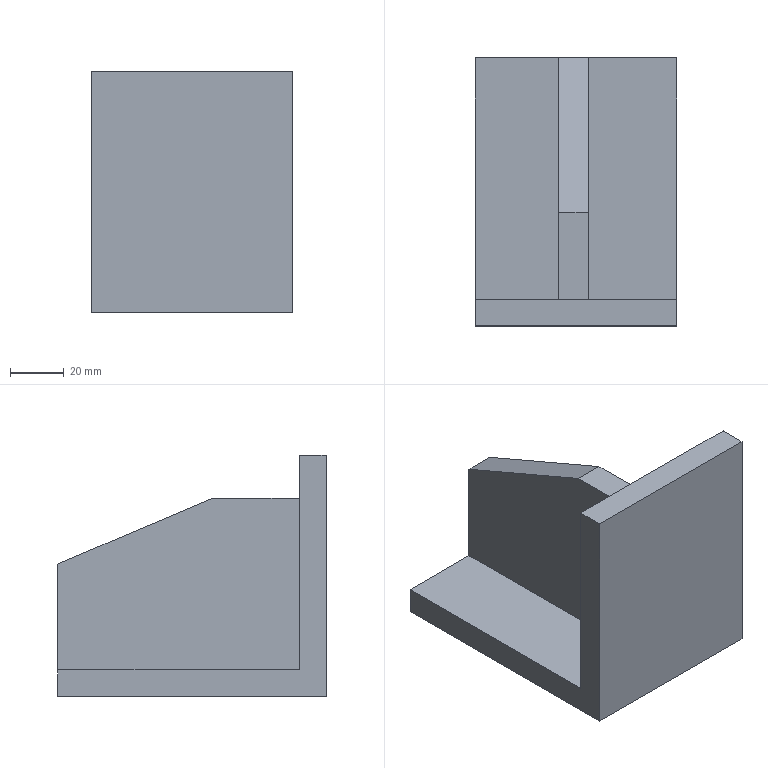Part | STEP file | MYT-A01-P39 | 1 solid | 13 faces | box 75 x 100 x 90 mm | volume 190302 mm3 | plane 13
STEP:
#1=CARTESIAN_POINT('',(-6.413,-40.,10.));
#2=VERTEX_POINT('',#1);
#3=CARTESIAN_POINT('',(-37.5,-40.,10.));
#4=VERTEX_POINT('',#3);
#5=CARTESIAN_POINT('',(-37.5,-40.,10.));
#6=DIRECTION('',(-1.,0.,0.));
#7=VECTOR('',#6,1000.);
#8=LINE('',#5,#7);
#9=EDGE_CURVE('',#2,#4,#8,.T.);
#10=ORIENTED_EDGE('',*,*,#9,.F.);
#11=CARTESIAN_POINT('',(-6.413,50.,10.));
#12=VERTEX_POINT('',#11);
#13=CARTESIAN_POINT('',(-6.413,50.,10.));
#14=DIRECTION('',(0.,-1.,0.));
#15=VECTOR('',#14,1000.);
#16=LINE('',#13,#15);
#17=EDGE_CURVE('',#12,#2,#16,.T.);
#18=ORIENTED_EDGE('',*,*,#17,.F.);
#19=CARTESIAN_POINT('',(-37.5,50.,10.));
#20=VERTEX_POINT('',#19);
#21=CARTESIAN_POINT('',(-37.5,50.,10.));
#22=DIRECTION('',(-1.,0.,0.));
#23=VECTOR('',#22,1000.);
#24=LINE('',#21,#23);
#25=EDGE_CURVE('',#12,#20,#24,.T.);
#26=ORIENTED_EDGE('',*,*,#25,.T.);
#27=CARTESIAN_POINT('',(-37.5,50.,10.));
#28=DIRECTION('',(0.,-1.,0.));
#29=VECTOR('',#28,1000.);
#30=LINE('',#27,#29);
#31=EDGE_CURVE('',#20,#4,#30,.T.);
#32=ORIENTED_EDGE('',*,*,#31,.T.);
#33=EDGE_LOOP('',(#10,#18,#26,#32));
#34=FACE_OUTER_BOUND('',#33,.T.);
#35=CARTESIAN_POINT('',(0.,0.,10.));
#36=DIRECTION('',(0.,0.,1.));
#37=DIRECTION('',(1.,0.,0.));
#38=AXIS2_PLACEMENT_3D('',#35,#36,#37);
#39=PLANE('',#38);
#40=ADVANCED_FACE('',(#34),#39,.T.);
#41=CARTESIAN_POINT('',(37.5,50.,10.));
#42=VERTEX_POINT('',#41);
#43=CARTESIAN_POINT('',(4.531,50.,10.));
#44=VERTEX_POINT('',#43);
#45=CARTESIAN_POINT('',(-37.5,50.,10.));
#46=DIRECTION('',(-1.,0.,0.));
#47=VECTOR('',#46,1000.);
#48=LINE('',#45,#47);
#49=EDGE_CURVE('',#42,#44,#48,.T.);
#50=ORIENTED_EDGE('',*,*,#49,.T.);
#51=CARTESIAN_POINT('',(4.531,-40.,10.));
#52=VERTEX_POINT('',#51);
#53=CARTESIAN_POINT('',(4.531,50.,10.));
#54=DIRECTION('',(0.,1.,0.));
#55=VECTOR('',#54,1000.);
#56=LINE('',#53,#55);
#57=EDGE_CURVE('',#52,#44,#56,.T.);
#58=ORIENTED_EDGE('',*,*,#57,.F.);
#59=CARTESIAN_POINT('',(37.5,-40.,10.));
#60=VERTEX_POINT('',#59);
#61=CARTESIAN_POINT('',(-37.5,-40.,10.));
#62=DIRECTION('',(-1.,0.,0.));
#63=VECTOR('',#62,1000.);
#64=LINE('',#61,#63);
#65=EDGE_CURVE('',#60,#52,#64,.T.);
#66=ORIENTED_EDGE('',*,*,#65,.F.);
#67=CARTESIAN_POINT('',(37.5,50.,10.));
#68=DIRECTION('',(0.,1.,0.));
#69=VECTOR('',#68,1000.);
#70=LINE('',#67,#69);
#71=EDGE_CURVE('',#60,#42,#70,.T.);
#72=ORIENTED_EDGE('',*,*,#71,.T.);
#73=EDGE_LOOP('',(#50,#58,#66,#72));
#74=FACE_OUTER_BOUND('',#73,.T.);
#75=CARTESIAN_POINT('',(0.,0.,10.));
#76=DIRECTION('',(0.,0.,1.));
#77=DIRECTION('',(1.,0.,0.));
#78=AXIS2_PLACEMENT_3D('',#75,#76,#77);
#79=PLANE('',#78);
#80=ADVANCED_FACE('',(#74),#79,.T.);
#81=CARTESIAN_POINT('',(-6.413,-40.,74.));
#82=VERTEX_POINT('',#81);
#83=CARTESIAN_POINT('',(-6.413,-40.,74.));
#84=DIRECTION('',(0.,0.,-1.));
#85=VECTOR('',#84,1000.);
#86=LINE('',#83,#85);
#87=EDGE_CURVE('',#82,#2,#86,.T.);
#88=ORIENTED_EDGE('',*,*,#87,.T.);
#89=ORIENTED_EDGE('',*,*,#9,.T.);
#90=CARTESIAN_POINT('',(-37.5,-40.,90.));
#91=VERTEX_POINT('',#90);
#92=CARTESIAN_POINT('',(-37.5,-40.,90.));
#93=DIRECTION('',(0.,0.,-1.));
#94=VECTOR('',#93,1000.);
#95=LINE('',#92,#94);
#96=EDGE_CURVE('',#91,#4,#95,.T.);
#97=ORIENTED_EDGE('',*,*,#96,.F.);
#98=CARTESIAN_POINT('',(37.5,-40.,90.));
#99=VERTEX_POINT('',#98);
#100=CARTESIAN_POINT('',(-37.5,-40.,90.));
#101=DIRECTION('',(-1.,0.,0.));
#102=VECTOR('',#101,1000.);
#103=LINE('',#100,#102);
#104=EDGE_CURVE('',#99,#91,#103,.T.);
#105=ORIENTED_EDGE('',*,*,#104,.F.);
#106=CARTESIAN_POINT('',(37.5,-40.,90.));
#107=DIRECTION('',(0.,0.,-1.));
#108=VECTOR('',#107,1000.);
#109=LINE('',#106,#108);
#110=EDGE_CURVE('',#99,#60,#109,.T.);
#111=ORIENTED_EDGE('',*,*,#110,.T.);
#112=ORIENTED_EDGE('',*,*,#65,.T.);
#113=CARTESIAN_POINT('',(4.531,-40.,74.));
#114=VERTEX_POINT('',#113);
#115=CARTESIAN_POINT('',(4.531,-40.,74.));
#116=DIRECTION('',(0.,0.,-1.));
#117=VECTOR('',#116,1000.);
#118=LINE('',#115,#117);
#119=EDGE_CURVE('',#114,#52,#118,.T.);
#120=ORIENTED_EDGE('',*,*,#119,.F.);
#121=CARTESIAN_POINT('',(-6.413,-40.,74.));
#122=DIRECTION('',(1.,0.,0.));
#123=VECTOR('',#122,1000.);
#124=LINE('',#121,#123);
#125=EDGE_CURVE('',#82,#114,#124,.T.);
#126=ORIENTED_EDGE('',*,*,#125,.F.);
#127=EDGE_LOOP('',(#88,#89,#97,#105,#111,#112,#120,#126));
#128=FACE_OUTER_BOUND('',#127,.T.);
#129=CARTESIAN_POINT('',(-37.5,-40.,90.));
#130=DIRECTION('',(0.,-1.,0.));
#131=DIRECTION('',(0.,0.,-1.));
#132=AXIS2_PLACEMENT_3D('',#129,#130,#131);
#133=PLANE('',#132);
#134=ADVANCED_FACE('',(#128),#133,.F.);
#135=CARTESIAN_POINT('',(37.5,-50.,0.));
#136=VERTEX_POINT('',#135);
#137=CARTESIAN_POINT('',(37.5,50.,0.));
#138=VERTEX_POINT('',#137);
#139=CARTESIAN_POINT('',(37.5,50.,0.));
#140=DIRECTION('',(0.,1.,0.));
#141=VECTOR('',#140,1000.);
#142=LINE('',#139,#141);
#143=EDGE_CURVE('',#136,#138,#142,.T.);
#144=ORIENTED_EDGE('',*,*,#143,.T.);
#145=CARTESIAN_POINT('',(37.5,50.,10.));
#146=DIRECTION('',(0.,0.,-1.));
#147=VECTOR('',#146,1000.);
#148=LINE('',#145,#147);
#149=EDGE_CURVE('',#42,#138,#148,.T.);
#150=ORIENTED_EDGE('',*,*,#149,.F.);
#151=ORIENTED_EDGE('',*,*,#71,.F.);
#152=ORIENTED_EDGE('',*,*,#110,.F.);
#153=CARTESIAN_POINT('',(37.5,-50.,90.));
#154=VERTEX_POINT('',#153);
#155=CARTESIAN_POINT('',(37.5,-50.,90.));
#156=DIRECTION('',(0.,1.,0.));
#157=VECTOR('',#156,1000.);
#158=LINE('',#155,#157);
#159=EDGE_CURVE('',#154,#99,#158,.T.);
#160=ORIENTED_EDGE('',*,*,#159,.F.);
#161=CARTESIAN_POINT('',(37.5,-50.,10.));
#162=DIRECTION('',(0.,0.,-1.));
#163=VECTOR('',#162,1000.);
#164=LINE('',#161,#163);
#165=EDGE_CURVE('',#154,#136,#164,.T.);
#166=ORIENTED_EDGE('',*,*,#165,.T.);
#167=EDGE_LOOP('',(#144,#150,#151,#152,#160,#166));
#168=FACE_OUTER_BOUND('',#167,.T.);
#169=CARTESIAN_POINT('',(37.5,50.,10.));
#170=DIRECTION('',(-1.,0.,0.));
#171=DIRECTION('',(0.,-1.,0.));
#172=AXIS2_PLACEMENT_3D('',#169,#170,#171);
#173=PLANE('',#172);
#174=ADVANCED_FACE('',(#168),#173,.F.);
#175=CARTESIAN_POINT('',(-6.413,50.,49.448));
#176=VERTEX_POINT('',#175);
#177=CARTESIAN_POINT('',(-6.413,50.,74.));
#178=DIRECTION('',(0.,0.,-1.));
#179=VECTOR('',#178,1000.);
#180=LINE('',#177,#179);
#181=EDGE_CURVE('',#176,#12,#180,.T.);
#182=ORIENTED_EDGE('',*,*,#181,.F.);
#183=CARTESIAN_POINT('',(4.531,50.,49.448));
#184=VERTEX_POINT('',#183);
#185=CARTESIAN_POINT('',(-37.5,50.,49.448));
#186=DIRECTION('',(1.,0.,0.));
#187=VECTOR('',#186,1000.);
#188=LINE('',#185,#187);
#189=EDGE_CURVE('',#176,#184,#188,.T.);
#190=ORIENTED_EDGE('',*,*,#189,.T.);
#191=CARTESIAN_POINT('',(4.531,50.,74.));
#192=DIRECTION('',(0.,0.,-1.));
#193=VECTOR('',#192,1000.);
#194=LINE('',#191,#193);
#195=EDGE_CURVE('',#184,#44,#194,.T.);
#196=ORIENTED_EDGE('',*,*,#195,.T.);
#197=ORIENTED_EDGE('',*,*,#49,.F.);
#198=ORIENTED_EDGE('',*,*,#149,.T.);
#199=CARTESIAN_POINT('',(-37.5,50.,0.));
#200=VERTEX_POINT('',#199);
#201=CARTESIAN_POINT('',(-37.5,50.,0.));
#202=DIRECTION('',(-1.,0.,0.));
#203=VECTOR('',#202,1000.);
#204=LINE('',#201,#203);
#205=EDGE_CURVE('',#138,#200,#204,.T.);
#206=ORIENTED_EDGE('',*,*,#205,.T.);
#207=CARTESIAN_POINT('',(-37.5,50.,10.));
#208=DIRECTION('',(0.,0.,-1.));
#209=VECTOR('',#208,1000.);
#210=LINE('',#207,#209);
#211=EDGE_CURVE('',#20,#200,#210,.T.);
#212=ORIENTED_EDGE('',*,*,#211,.F.);
#213=ORIENTED_EDGE('',*,*,#25,.F.);
#214=EDGE_LOOP('',(#182,#190,#196,#197,#198,#206,#212,#213));
#215=FACE_OUTER_BOUND('',#214,.T.);
#216=CARTESIAN_POINT('',(-37.5,50.,10.));
#217=DIRECTION('',(0.,-1.,0.));
#218=DIRECTION('',(0.,0.,-1.));
#219=AXIS2_PLACEMENT_3D('',#216,#217,#218);
#220=PLANE('',#219);
#221=ADVANCED_FACE('',(#215),#220,.F.);
#222=CARTESIAN_POINT('',(-37.5,-50.,0.));
#223=VERTEX_POINT('',#222);
#224=CARTESIAN_POINT('',(-37.5,50.,0.));
#225=DIRECTION('',(0.,-1.,0.));
#226=VECTOR('',#225,1000.);
#227=LINE('',#224,#226);
#228=EDGE_CURVE('',#200,#223,#227,.T.);
#229=ORIENTED_EDGE('',*,*,#228,.T.);
#230=CARTESIAN_POINT('',(-37.5,-50.,90.));
#231=VERTEX_POINT('',#230);
#232=CARTESIAN_POINT('',(-37.5,-50.,10.));
#233=DIRECTION('',(0.,0.,-1.));
#234=VECTOR('',#233,1000.);
#235=LINE('',#232,#234);
#236=EDGE_CURVE('',#231,#223,#235,.T.);
#237=ORIENTED_EDGE('',*,*,#236,.F.);
#238=CARTESIAN_POINT('',(-37.5,-50.,90.));
#239=DIRECTION('',(0.,-1.,0.));
#240=VECTOR('',#239,1000.);
#241=LINE('',#238,#240);
#242=EDGE_CURVE('',#91,#231,#241,.T.);
#243=ORIENTED_EDGE('',*,*,#242,.F.);
#244=ORIENTED_EDGE('',*,*,#96,.T.);
#245=ORIENTED_EDGE('',*,*,#31,.F.);
#246=ORIENTED_EDGE('',*,*,#211,.T.);
#247=EDGE_LOOP('',(#229,#237,#243,#244,#245,#246));
#248=FACE_OUTER_BOUND('',#247,.T.);
#249=CARTESIAN_POINT('',(-37.5,50.,10.));
#250=DIRECTION('',(1.,0.,0.));
#251=DIRECTION('',(0.,1.,0.));
#252=AXIS2_PLACEMENT_3D('',#249,#250,#251);
#253=PLANE('',#252);
#254=ADVANCED_FACE('',(#248),#253,.F.);
#255=CARTESIAN_POINT('',(-37.5,-50.,0.));
#256=DIRECTION('',(1.,0.,0.));
#257=VECTOR('',#256,1000.);
#258=LINE('',#255,#257);
#259=EDGE_CURVE('',#223,#136,#258,.T.);
#260=ORIENTED_EDGE('',*,*,#259,.T.);
#261=ORIENTED_EDGE('',*,*,#165,.F.);
#262=CARTESIAN_POINT('',(-37.5,-50.,90.));
#263=DIRECTION('',(1.,0.,0.));
#264=VECTOR('',#263,1000.);
#265=LINE('',#262,#264);
#266=EDGE_CURVE('',#231,#154,#265,.T.);
#267=ORIENTED_EDGE('',*,*,#266,.F.);
#268=ORIENTED_EDGE('',*,*,#236,.T.);
#269=EDGE_LOOP('',(#260,#261,#267,#268));
#270=FACE_OUTER_BOUND('',#269,.T.);
#271=CARTESIAN_POINT('',(-37.5,-50.,10.));
#272=DIRECTION('',(0.,1.,0.));
#273=DIRECTION('',(0.,0.,1.));
#274=AXIS2_PLACEMENT_3D('',#271,#272,#273);
#275=PLANE('',#274);
#276=ADVANCED_FACE('',(#270),#275,.F.);
#277=ORIENTED_EDGE('',*,*,#143,.F.);
#278=ORIENTED_EDGE('',*,*,#259,.F.);
#279=ORIENTED_EDGE('',*,*,#228,.F.);
#280=ORIENTED_EDGE('',*,*,#205,.F.);
#281=EDGE_LOOP('',(#277,#278,#279,#280));
#282=FACE_OUTER_BOUND('',#281,.T.);
#283=CARTESIAN_POINT('',(0.,0.,0.));
#284=DIRECTION('',(0.,0.,1.));
#285=DIRECTION('',(1.,0.,0.));
#286=AXIS2_PLACEMENT_3D('',#283,#284,#285);
#287=PLANE('',#286);
#288=ADVANCED_FACE('',(#282),#287,.F.);
#289=ORIENTED_EDGE('',*,*,#242,.T.);
#290=ORIENTED_EDGE('',*,*,#266,.T.);
#291=ORIENTED_EDGE('',*,*,#159,.T.);
#292=ORIENTED_EDGE('',*,*,#104,.T.);
#293=EDGE_LOOP('',(#289,#290,#291,#292));
#294=FACE_OUTER_BOUND('',#293,.T.);
#295=CARTESIAN_POINT('',(0.,0.,90.));
#296=DIRECTION('',(0.,0.,-1.));
#297=DIRECTION('',(-1.,0.,0.));
#298=AXIS2_PLACEMENT_3D('',#295,#296,#297);
#299=PLANE('',#298);
#300=ADVANCED_FACE('',(#294),#299,.F.);
#301=CARTESIAN_POINT('',(-6.413,-7.581,74.));
#302=VERTEX_POINT('',#301);
#303=CARTESIAN_POINT('',(-6.413,50.,74.));
#304=DIRECTION('',(0.,-1.,0.));
#305=VECTOR('',#304,1000.);
#306=LINE('',#303,#305);
#307=EDGE_CURVE('',#302,#82,#306,.T.);
#308=ORIENTED_EDGE('',*,*,#307,.F.);
#309=CARTESIAN_POINT('',(-6.413,71.812,40.147));
#310=DIRECTION('',(0.,-0.9199,0.3922));
#311=VECTOR('',#310,1000.);
#312=LINE('',#309,#311);
#313=EDGE_CURVE('',#176,#302,#312,.T.);
#314=ORIENTED_EDGE('',*,*,#313,.F.);
#315=ORIENTED_EDGE('',*,*,#181,.T.);
#316=ORIENTED_EDGE('',*,*,#17,.T.);
#317=ORIENTED_EDGE('',*,*,#87,.F.);
#318=EDGE_LOOP('',(#308,#314,#315,#316,#317));
#319=FACE_OUTER_BOUND('',#318,.T.);
#320=CARTESIAN_POINT('',(-6.413,50.,74.));
#321=DIRECTION('',(1.,0.,0.));
#322=DIRECTION('',(0.,0.,-1.));
#323=AXIS2_PLACEMENT_3D('',#320,#321,#322);
#324=PLANE('',#323);
#325=ADVANCED_FACE('',(#319),#324,.F.);
#326=ORIENTED_EDGE('',*,*,#195,.F.);
#327=CARTESIAN_POINT('',(4.531,-7.581,74.));
#328=VERTEX_POINT('',#327);
#329=CARTESIAN_POINT('',(4.531,41.142,53.225));
#330=DIRECTION('',(0.,-0.9199,0.3922));
#331=VECTOR('',#330,1000.);
#332=LINE('',#329,#331);
#333=EDGE_CURVE('',#184,#328,#332,.T.);
#334=ORIENTED_EDGE('',*,*,#333,.T.);
#335=CARTESIAN_POINT('',(4.531,50.,74.));
#336=DIRECTION('',(0.,1.,0.));
#337=VECTOR('',#336,1000.);
#338=LINE('',#335,#337);
#339=EDGE_CURVE('',#114,#328,#338,.T.);
#340=ORIENTED_EDGE('',*,*,#339,.F.);
#341=ORIENTED_EDGE('',*,*,#119,.T.);
#342=ORIENTED_EDGE('',*,*,#57,.T.);
#343=EDGE_LOOP('',(#326,#334,#340,#341,#342));
#344=FACE_OUTER_BOUND('',#343,.T.);
#345=CARTESIAN_POINT('',(4.531,50.,74.));
#346=DIRECTION('',(-1.,0.,0.));
#347=DIRECTION('',(0.,0.,1.));
#348=AXIS2_PLACEMENT_3D('',#345,#346,#347);
#349=PLANE('',#348);
#350=ADVANCED_FACE('',(#344),#349,.F.);
#351=CARTESIAN_POINT('',(0.,-7.581,74.));
#352=DIRECTION('',(1.,0.,0.));
#353=VECTOR('',#352,1000.);
#354=LINE('',#351,#353);
#355=EDGE_CURVE('',#302,#328,#354,.T.);
#356=ORIENTED_EDGE('',*,*,#355,.F.);
#357=ORIENTED_EDGE('',*,*,#307,.T.);
#358=ORIENTED_EDGE('',*,*,#125,.T.);
#359=ORIENTED_EDGE('',*,*,#339,.T.);
#360=EDGE_LOOP('',(#356,#357,#358,#359));
#361=FACE_OUTER_BOUND('',#360,.T.);
#362=CARTESIAN_POINT('',(0.,0.,74.));
#363=DIRECTION('',(0.,0.,1.));
#364=DIRECTION('',(1.,0.,0.));
#365=AXIS2_PLACEMENT_3D('',#362,#363,#364);
#366=PLANE('',#365);
#367=ADVANCED_FACE('',(#361),#366,.T.);
#368=ORIENTED_EDGE('',*,*,#313,.T.);
#369=ORIENTED_EDGE('',*,*,#355,.T.);
#370=ORIENTED_EDGE('',*,*,#333,.F.);
#371=ORIENTED_EDGE('',*,*,#189,.F.);
#372=EDGE_LOOP('',(#368,#369,#370,#371));
#373=FACE_OUTER_BOUND('',#372,.T.);
#374=CARTESIAN_POINT('',(57.587,71.812,40.147));
#375=DIRECTION('',(0.,-0.3922,-0.9199));
#376=DIRECTION('',(0.,0.9199,-0.3922));
#377=AXIS2_PLACEMENT_3D('',#374,#375,#376);
#378=PLANE('',#377);
#379=ADVANCED_FACE('',(#373),#378,.F.);
#380=CLOSED_SHELL('',(#40,#80,#134,#174,#221,#254,#276,#288,#300,#325,#350,#367,#379));
#381=MANIFOLD_SOLID_BREP('',#380);
#382=CARTESIAN_POINT('',(0.,0.,0.));
#383=DIRECTION('',(0.,0.,1.));
#384=DIRECTION('',(1.,0.,0.));
#385=AXIS2_PLACEMENT_3D('',#382,#383,#384);
#386=(LENGTH_UNIT()NAMED_UNIT(*)SI_UNIT(.MILLI.,.METRE.));
#387=UNCERTAINTY_MEASURE_WITH_UNIT(LENGTH_MEASURE(0.00001),#386,'','');
#388=(NAMED_UNIT(*)PLANE_ANGLE_UNIT()SI_UNIT($,.RADIAN.));
#389=(NAMED_UNIT(*)SI_UNIT($,.STERADIAN.)SOLID_ANGLE_UNIT());
#390=(GEOMETRIC_REPRESENTATION_CONTEXT(3)GLOBAL_UNCERTAINTY_ASSIGNED_CONTEXT((#387))GLOBAL_UNIT_ASSIGNED_CONTEXT((#386,#388,#389))REPRESENTATION_CONTEXT('',''));
#391=ADVANCED_BREP_SHAPE_REPRESENTATION('',(#381,#385),#390);